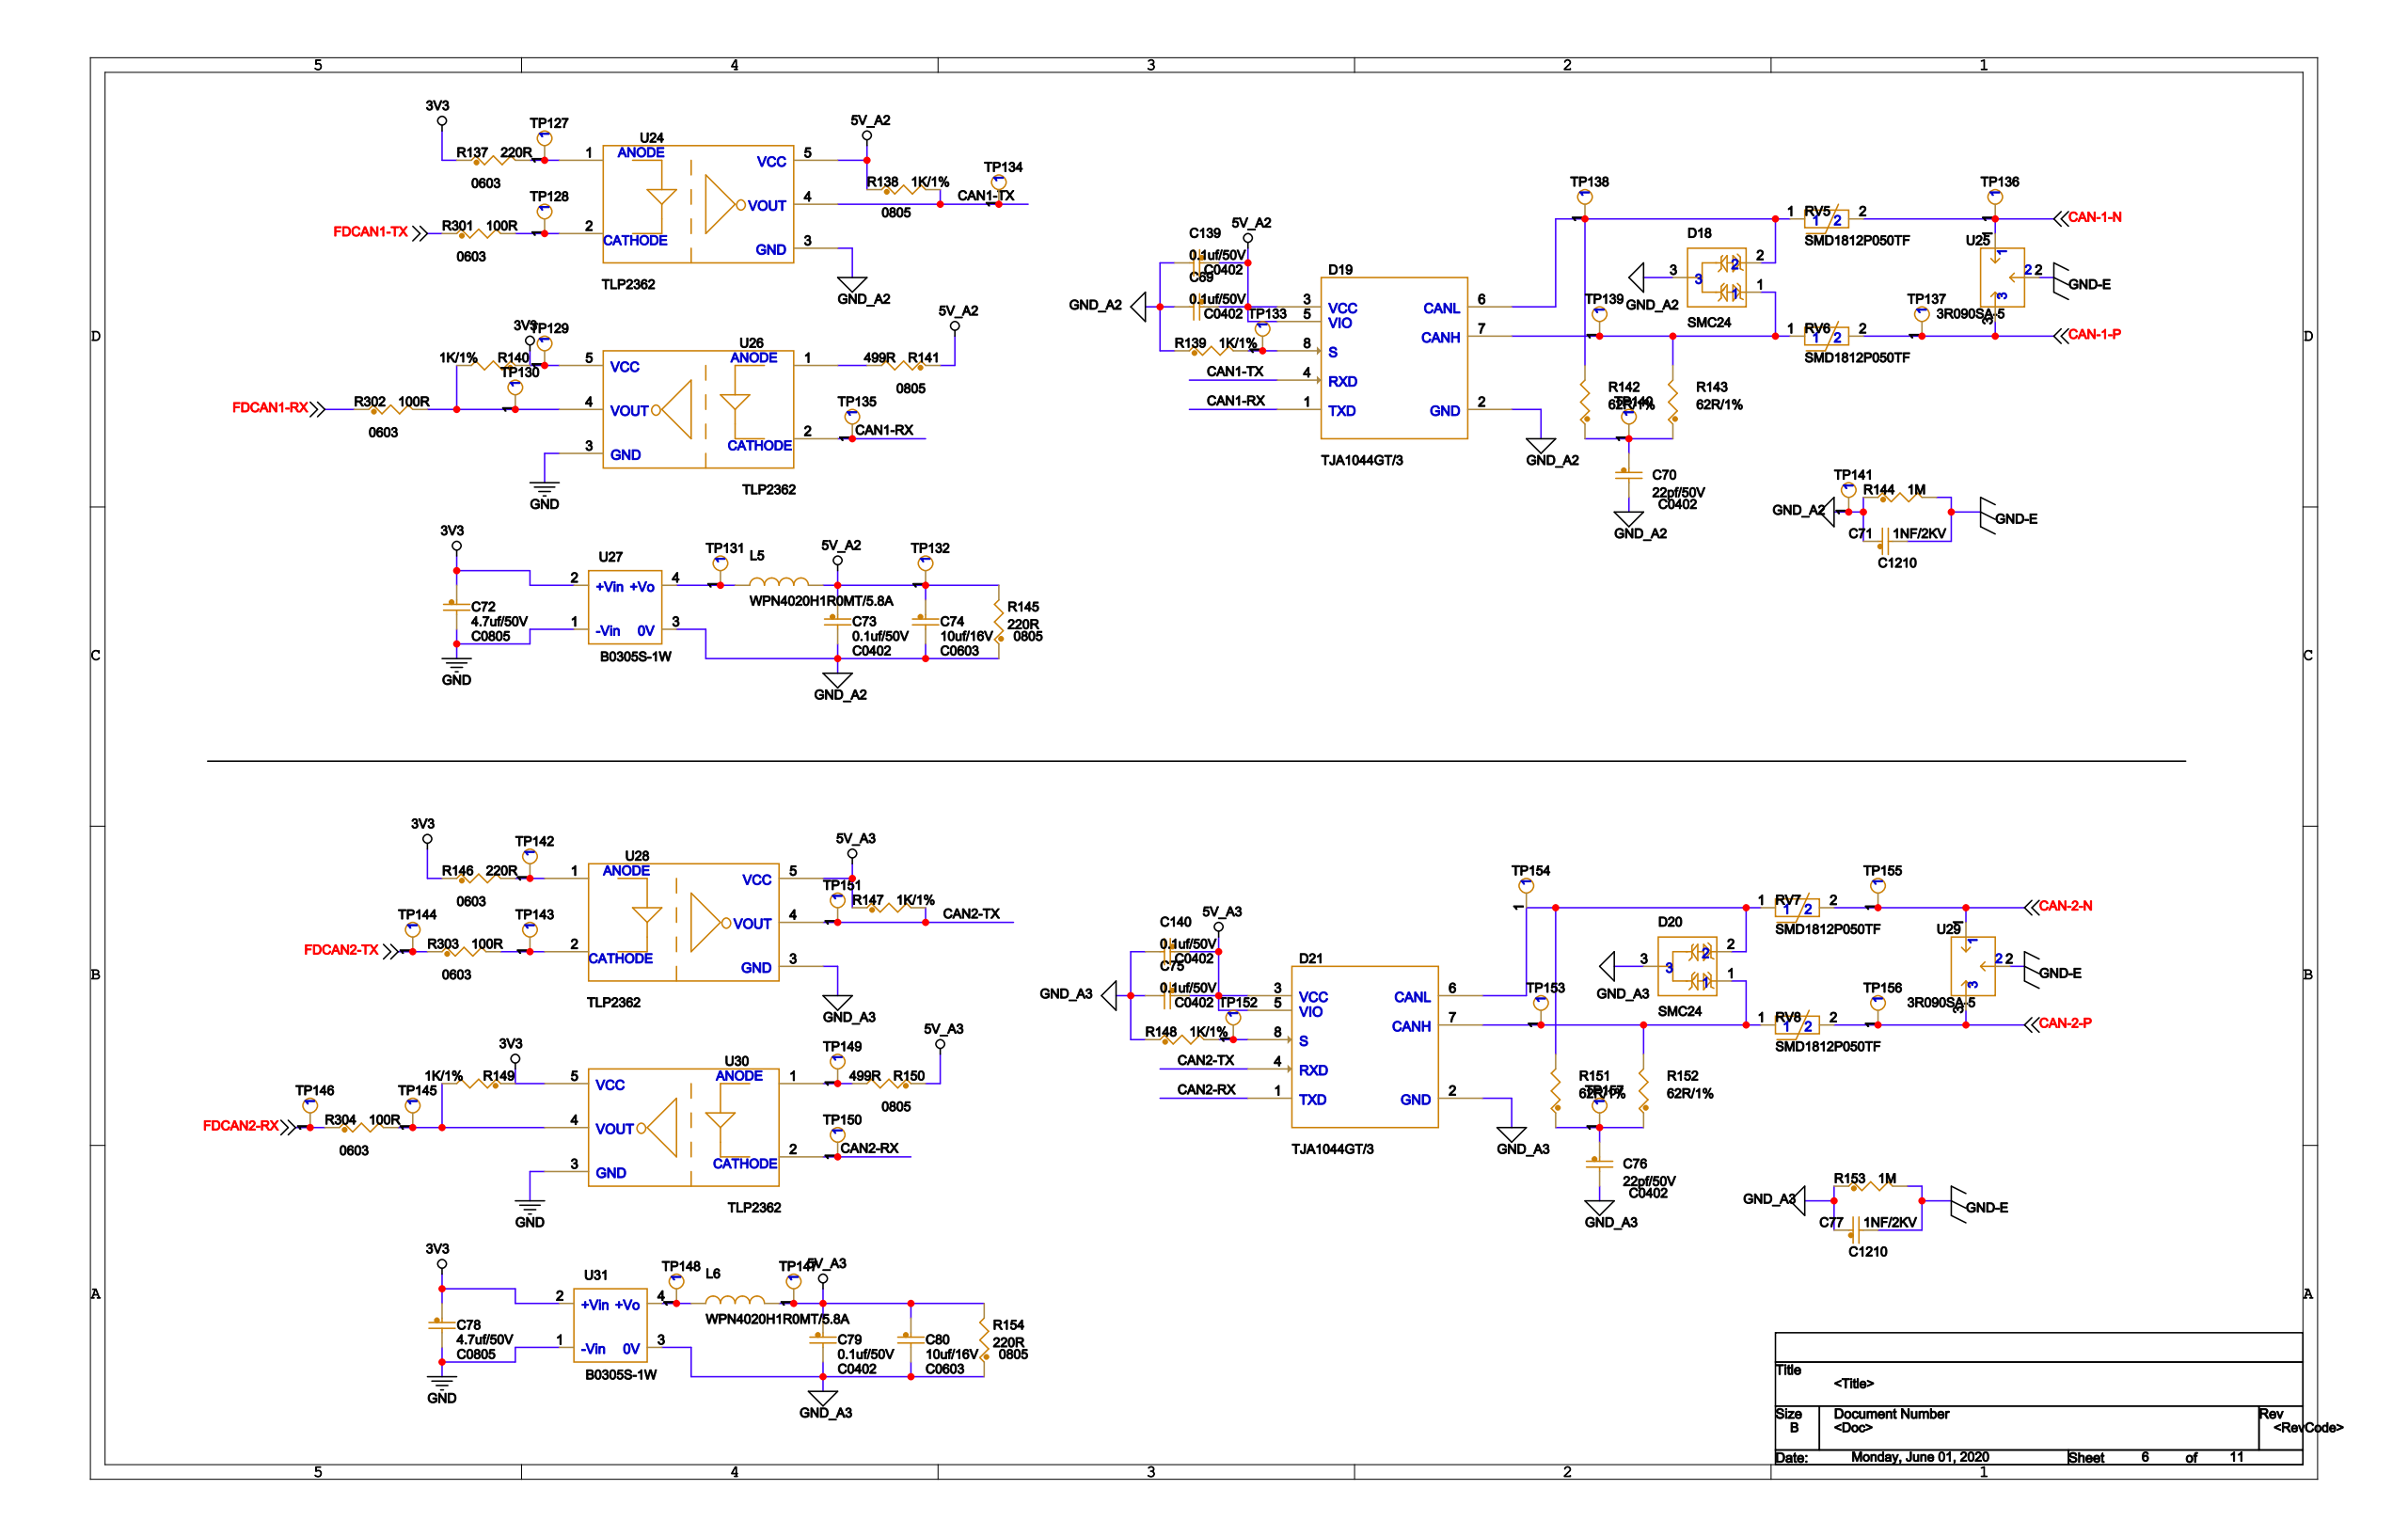Circuit board | Cadence Allegro | 792 parts | 400 nets | one sheet of the schematic
Parts on this sheet (reference | value | footprint):
C69 | 0.1uf/50V | C0402
C70 | 22pf/50V | C0402
C71 | 1NF/2KV | C1210
C72 | 4.7uf/50V | C0805
C73 | 0.1uf/50V | C0402
C74 | 10uf/16V | C0603
C75 | 0.1uf/50V | C0402
C76 | 22pf/50V | C0402
C77 | 1NF/2KV | C1210
C78 | 4.7uf/50V | C0805
C79 | 0.1uf/50V | C0402
C80 | 10uf/16V | C0603
C139 | 0.1uf/50V | C0402
C140 | 0.1uf/50V | C0402
D18 | SMC24 | SOT23
D19 | TJA1044GT/3 | SO8
D20 | SMC24 | SOT23
D21 | TJA1044GT/3 | SO8
L5 | WPN4020H1R0MT/5.8A | SM_IND_4
L6 | WPN4020H1R0MT/5.8A | SM_IND_4
R137 | 220R | 0603
R138 | 1K/1% | 0805
R139 | 1K/1% | 0603
R140 | 1K/1% | 0603
R141 | 499R | 0805
R142 | 62R/1% | 1206
R143 | 62R/1% | 1206
R144 | 1M | 1206
R145 | 220R | 0805
R146 | 220R | 0603
R147 | 1K/1% | 0805
R148 | 1K/1% | 0603
R149 | 1K/1% | 0603
R150 | 499R | 0805
R151 | 62R/1% | 1206
R152 | 62R/1% | 1206
R153 | 1M | 1206
R154 | 220R | 0805
R301 | 100R | 0603
R302 | 100R | 0603
R303 | 100R | 0603
R304 | 100R | 0603
RV5 | SMD1812P050TF | 1812_2
RV6 | SMD1812P050TF | 1812_2
RV7 | SMD1812P050TF | 1812_2
RV8 | SMD1812P050TF | 1812_2
TP127 | TESTPOINT | TESTPOINT-33MIL
TP128 | TESTPOINT | TESTPOINT-33MIL
TP129 | TESTPOINT | TESTPOINT-33MIL
TP130 | TESTPOINT | TESTPOINT-33MIL
TP131 | TESTPOINT | TESTPOINT-33MIL
TP132 | TESTPOINT | TESTPOINT-33MIL
TP133 | TESTPOINT | TESTPOINT-33MIL
TP134 | TESTPOINT | TESTPOINT-33MIL
TP135 | TESTPOINT | TESTPOINT-33MIL
TP136 | TESTPOINT | TESTPOINT-33MIL
TP137 | TESTPOINT | TESTPOINT-33MIL
TP138 | TESTPOINT | TESTPOINT-33MIL
TP139 | TESTPOINT | TESTPOINT-33MIL
TP140 | TESTPOINT | TESTPOINT-33MIL
TP141 | TESTPOINT | TESTPOINT-33MIL
TP142 | TESTPOINT | TESTPOINT-33MIL
TP143 | TESTPOINT | TESTPOINT-33MIL
TP144 | TESTPOINT | TESTPOINT-33MIL
TP145 | TESTPOINT | TESTPOINT-33MIL
TP146 | TESTPOINT | TESTPOINT-33MIL
TP147 | TESTPOINT | TESTPOINT-33MIL
TP148 | TESTPOINT | TESTPOINT-33MIL
TP149 | TESTPOINT | TESTPOINT-33MIL
TP150 | TESTPOINT | TESTPOINT-33MIL
TP151 | TESTPOINT | TESTPOINT-33MIL
TP152 | TESTPOINT | TESTPOINT-33MIL
TP153 | TESTPOINT | TESTPOINT-33MIL
TP154 | TESTPOINT | TESTPOINT-33MIL
TP155 | TESTPOINT | TESTPOINT-33MIL
TP156 | TESTPOINT | TESTPOINT-33MIL
TP157 | TESTPOINT | TESTPOINT-33MIL
U24 | TLP2362 | TLP2362
U25 | 3R090SA-5 | 3R090SA-5
U26 | TLP2362 | TLP2362
U27 | B0305S-1W | B0303S
U28 | TLP2362 | TLP2362
U29 | 3R090SA-5 | 3R090SA-5
U30 | TLP2362 | TLP2362
U31 | B0305S-1W | B0303S
Nets of these parts (net: part-pin ...):
3V3: C72-1 C78-1 R137-1 R140-1 R146-1 R149-1 TP129-1 U26-5 U27-2 U30-5 U31-2
GND-E: C71-2 C77-2 R144-2 R153-2 U25-2 U29-2
GND: C72-2 C78-2 U26-3 U27-1 U30-3 U31-1
CAN-1-P: RV6-2 TP137-1 U25-3
CAN-1-N: RV5-2 TP136-1 U25-1
N7247638: R137-2 TP127-1 U24-1
N7247642: R301-2 TP128-1 U24-2
N7247810: R140-2 R302-2 TP130-1 U26-4
N7248108: L5-1 TP131-1 U27-4
5V_A2: C69-1 C73-1 C74-1 C139-1 D19-3 D19-5 L5-2 R138-1 R141-1 R145-2 TP132-1 U24-5
N7843129: D19-8 R139-2 TP133-1
CAN1-TX: D19-4 R138-2 TP134-1 U24-4
CAN1-RX: D19-1 TP135-1 U26-2
N7247038: D18-2 D19-6 R142-2 RV5-1 TP138-1
N7247046: D18-1 D19-7 R143-2 RV6-1 TP139-1
N7250475: C70-1 R142-1 R143-1 TP140-1
GND_A2: C69-2 C70-2 C71-1 C73-2 C74-2 C139-2 D18-3 D19-2 R139-1 R144-1 R145-1 TP141-1 U24-3 U27-3
N7252703: R146-2 TP142-1 U28-1
N7252707: R303-2 TP143-1 U28-2
FDCAN2-TX: R303-1 TP144-1
N7252749: R149-2 R304-2 TP145-1 U30-4
FDCAN2-RX: R304-1 TP146-1
5V_A3: C75-1 C79-1 C80-1 C140-1 D21-3 D21-5 L6-2 R147-1 R150-1 R154-2 TP147-1 U28-5
N7253075: L6-1 TP148-1 U31-4
N7252789: R150-2 TP149-1 U30-1
CAN2-RX: D21-1 TP150-1 U30-2
CAN2-TX: D21-4 R147-2 TP151-1 U28-4
N7843864: D21-8 R148-2 TP152-1
N7252227: D20-1 D21-7 R152-2 RV8-1 TP153-1
N7252219: D20-2 D21-6 R151-2 RV7-1 TP154-1
CAN-2-N: RV7-2 TP155-1 U29-1
CAN-2-P: RV8-2 TP156-1 U29-3
N7252251: C76-1 R151-1 R152-1 TP157-1
FDCAN1-RX: R302-1
FDCAN1-TX: R301-1
N7247776: R141-2 U26-1
GND_A3: C75-2 C76-2 C77-1 C79-2 C80-2 C140-2 D20-3 D21-2 R148-1 R153-1 R154-1 U28-3 U31-3